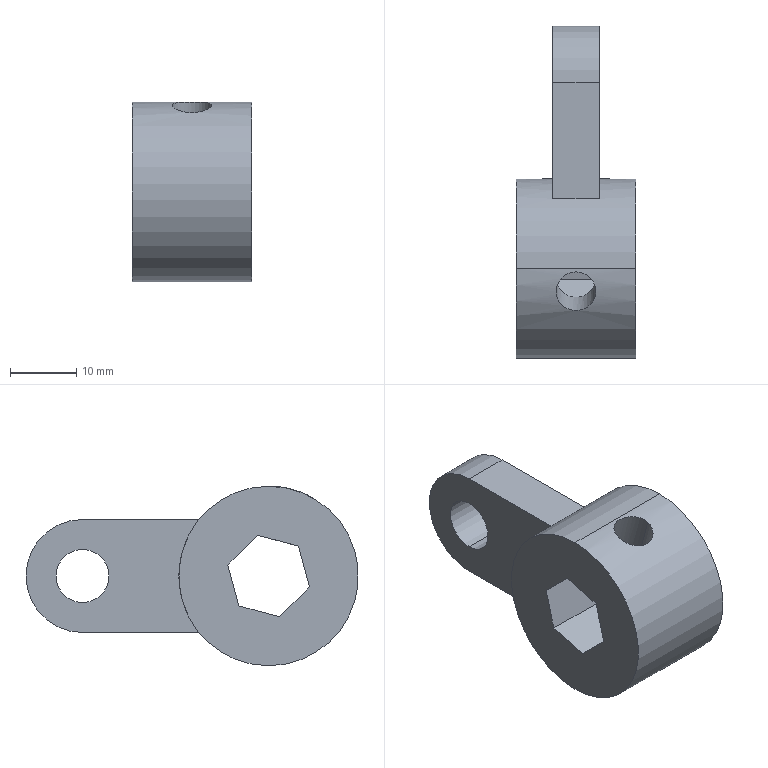Part | NX | features BREP 1 | 1 solid | 19 faces | box 18 x 50 x 27 mm | volume 10478 mm3 | plane 12 | cylinder 7 | commonest cylinder face diameters 6 x2 8 x2 27 x2 17 x1
STEP:
#1=CARTESIAN_POINT('',(-9.,0.,13.5));
#2=VERTEX_POINT('',#1);
#3=CARTESIAN_POINT('',(-9.,0.,-13.5));
#4=VERTEX_POINT('',#3);
#5=CARTESIAN_POINT('',(-9.,0.,0.));
#6=DIRECTION('',(1.,0.,0.));
#7=DIRECTION('',(0.,0.,1.));
#8=AXIS2_PLACEMENT_3D('',#5,#6,#7);
#9=CIRCLE('',#8,13.5);
#10=EDGE_CURVE('',#2,#4,#9,.T.);
#11=ORIENTED_EDGE('',*,*,#10,.F.);
#12=CARTESIAN_POINT('',(-9.,0.,0.));
#13=DIRECTION('',(1.,0.,0.));
#14=DIRECTION('',(0.,0.,-1.));
#15=AXIS2_PLACEMENT_3D('',#12,#13,#14);
#16=CIRCLE('',#15,13.5);
#17=EDGE_CURVE('',#4,#2,#16,.T.);
#18=ORIENTED_EDGE('',*,*,#17,.F.);
#19=EDGE_LOOP('',(#11,#18));
#20=FACE_BOUND('',#19,.T.);
#21=CARTESIAN_POINT('',(-9.,-4.491,4.491));
#22=VERTEX_POINT('',#21);
#23=CARTESIAN_POINT('',(-9.,-6.134,-1.644));
#24=VERTEX_POINT('',#23);
#25=CARTESIAN_POINT('',(-9.,-4.491,4.491));
#26=DIRECTION('',(0.,-0.2588,-0.9659));
#27=VECTOR('',#26,1000.);
#28=LINE('',#25,#27);
#29=EDGE_CURVE('',#22,#24,#28,.T.);
#30=ORIENTED_EDGE('',*,*,#29,.T.);
#31=CARTESIAN_POINT('',(-9.,-1.644,-6.134));
#32=VERTEX_POINT('',#31);
#33=CARTESIAN_POINT('',(-9.,-6.134,-1.644));
#34=DIRECTION('',(0.,0.7071,-0.7071));
#35=VECTOR('',#34,1000.);
#36=LINE('',#33,#35);
#37=EDGE_CURVE('',#24,#32,#36,.T.);
#38=ORIENTED_EDGE('',*,*,#37,.T.);
#39=CARTESIAN_POINT('',(-9.,4.491,-4.491));
#40=VERTEX_POINT('',#39);
#41=CARTESIAN_POINT('',(-9.,-1.644,-6.134));
#42=DIRECTION('',(0.,0.9659,0.2588));
#43=VECTOR('',#42,1000.);
#44=LINE('',#41,#43);
#45=EDGE_CURVE('',#32,#40,#44,.T.);
#46=ORIENTED_EDGE('',*,*,#45,.T.);
#47=CARTESIAN_POINT('',(-9.,6.134,1.644));
#48=VERTEX_POINT('',#47);
#49=CARTESIAN_POINT('',(-9.,4.491,-4.491));
#50=DIRECTION('',(0.,0.2588,0.9659));
#51=VECTOR('',#50,1000.);
#52=LINE('',#49,#51);
#53=EDGE_CURVE('',#40,#48,#52,.T.);
#54=ORIENTED_EDGE('',*,*,#53,.T.);
#55=CARTESIAN_POINT('',(-9.,1.644,6.134));
#56=VERTEX_POINT('',#55);
#57=CARTESIAN_POINT('',(-9.,6.134,1.644));
#58=DIRECTION('',(0.,-0.7071,0.7071));
#59=VECTOR('',#58,1000.);
#60=LINE('',#57,#59);
#61=EDGE_CURVE('',#48,#56,#60,.T.);
#62=ORIENTED_EDGE('',*,*,#61,.T.);
#63=CARTESIAN_POINT('',(-9.,1.644,6.134));
#64=DIRECTION('',(0.,-0.9659,-0.2588));
#65=VECTOR('',#64,1000.);
#66=LINE('',#63,#65);
#67=EDGE_CURVE('',#56,#22,#66,.T.);
#68=ORIENTED_EDGE('',*,*,#67,.T.);
#69=EDGE_LOOP('',(#30,#38,#46,#54,#62,#68));
#70=FACE_BOUND('',#69,.T.);
#71=CARTESIAN_POINT('',(-9.,0.,0.));
#72=DIRECTION('',(1.,0.,0.));
#73=DIRECTION('',(0.,1.,0.));
#74=AXIS2_PLACEMENT_3D('',#71,#72,#73);
#75=PLANE('',#74);
#76=ADVANCED_FACE('',(#20,#70),#75,.F.);
#77=CARTESIAN_POINT('',(9.,0.,13.5));
#78=VERTEX_POINT('',#77);
#79=CARTESIAN_POINT('',(-9.,0.,13.5));
#80=DIRECTION('',(1.,0.,0.));
#81=VECTOR('',#80,1000.);
#82=LINE('',#79,#81);
#83=EDGE_CURVE('',#78,#2,#82,.F.);
#84=ORIENTED_EDGE('',*,*,#83,.F.);
#85=CARTESIAN_POINT('',(9.,0.,-13.5));
#86=VERTEX_POINT('',#85);
#87=CARTESIAN_POINT('',(9.,0.,0.));
#88=DIRECTION('',(1.,0.,0.));
#89=DIRECTION('',(0.,0.,-1.));
#90=AXIS2_PLACEMENT_3D('',#87,#88,#89);
#91=CIRCLE('',#90,13.5);
#92=EDGE_CURVE('',#86,#78,#91,.T.);
#93=ORIENTED_EDGE('',*,*,#92,.F.);
#94=CARTESIAN_POINT('',(-9.,0.,-13.5));
#95=DIRECTION('',(1.,0.,0.));
#96=VECTOR('',#95,1000.);
#97=LINE('',#94,#96);
#98=EDGE_CURVE('',#86,#4,#97,.F.);
#99=ORIENTED_EDGE('',*,*,#98,.T.);
#100=ORIENTED_EDGE('',*,*,#17,.T.);
#101=EDGE_LOOP('',(#84,#93,#99,#100));
#102=FACE_BOUND('',#101,.T.);
#103=CARTESIAN_POINT('',(3.5,10.488,-8.5));
#104=VERTEX_POINT('',#103);
#105=CARTESIAN_POINT('',(3.5,10.488,8.5));
#106=VERTEX_POINT('',#105);
#107=CARTESIAN_POINT('',(3.5,0.,0.));
#108=DIRECTION('',(1.,0.,0.));
#109=DIRECTION('',(0.,0.7769,-0.6296));
#110=AXIS2_PLACEMENT_3D('',#107,#108,#109);
#111=CIRCLE('',#110,13.5);
#112=EDGE_CURVE('',#104,#106,#111,.T.);
#113=ORIENTED_EDGE('',*,*,#112,.T.);
#114=CARTESIAN_POINT('',(-3.5,10.488,8.5));
#115=VERTEX_POINT('',#114);
#116=CARTESIAN_POINT('',(-3.5,10.488,8.5));
#117=DIRECTION('',(1.,0.,0.));
#118=VECTOR('',#117,1000.);
#119=LINE('',#116,#118);
#120=EDGE_CURVE('',#115,#106,#119,.T.);
#121=ORIENTED_EDGE('',*,*,#120,.F.);
#122=CARTESIAN_POINT('',(-3.5,10.488,-8.5));
#123=VERTEX_POINT('',#122);
#124=CARTESIAN_POINT('',(-3.5,0.,0.));
#125=DIRECTION('',(1.,0.,0.));
#126=DIRECTION('',(0.,0.7769,-0.6296));
#127=AXIS2_PLACEMENT_3D('',#124,#125,#126);
#128=CIRCLE('',#127,13.5);
#129=EDGE_CURVE('',#123,#115,#128,.T.);
#130=ORIENTED_EDGE('',*,*,#129,.F.);
#131=CARTESIAN_POINT('',(-3.5,10.488,-8.5));
#132=DIRECTION('',(1.,0.,0.));
#133=VECTOR('',#132,1000.);
#134=LINE('',#131,#133);
#135=EDGE_CURVE('',#123,#104,#134,.T.);
#136=ORIENTED_EDGE('',*,*,#135,.T.);
#137=EDGE_LOOP('',(#113,#121,#130,#136));
#138=FACE_BOUND('',#137,.T.);
#139=CARTESIAN_POINT('',(-9.,0.,0.));
#140=DIRECTION('',(1.,0.,0.));
#141=DIRECTION('',(0.,0.,-1.));
#142=AXIS2_PLACEMENT_3D('',#139,#140,#141);
#143=CYLINDRICAL_SURFACE('',#142,13.5);
#144=ADVANCED_FACE('',(#102,#138),#143,.T.);
#145=ORIENTED_EDGE('',*,*,#98,.F.);
#146=CARTESIAN_POINT('',(9.,0.,0.));
#147=DIRECTION('',(1.,0.,0.));
#148=DIRECTION('',(0.,0.,1.));
#149=AXIS2_PLACEMENT_3D('',#146,#147,#148);
#150=CIRCLE('',#149,13.5);
#151=EDGE_CURVE('',#78,#86,#150,.T.);
#152=ORIENTED_EDGE('',*,*,#151,.F.);
#153=ORIENTED_EDGE('',*,*,#83,.T.);
#154=ORIENTED_EDGE('',*,*,#10,.T.);
#155=EDGE_LOOP('',(#145,#152,#153,#154));
#156=FACE_BOUND('',#155,.T.);
#157=CARTESIAN_POINT('',(-3.,-3.494,13.04));
#158=VERTEX_POINT('',#157);
#159=CARTESIAN_POINT('',(3.,-3.494,13.04));
#160=VERTEX_POINT('',#159);
#161=CARTESIAN_POINT('',(-3.,-3.494,13.04));
#162=CARTESIAN_POINT('',(-3.,-2.73,13.245));
#163=CARTESIAN_POINT('',(-2.352,-1.186,13.486));
#164=CARTESIAN_POINT('',(0.0001371,-0.1703,13.492));
#165=CARTESIAN_POINT('',(2.354,-1.187,13.486));
#166=CARTESIAN_POINT('',(3.,-2.732,13.244));
#167=CARTESIAN_POINT('',(3.,-3.494,13.04));
#168=B_SPLINE_CURVE_WITH_KNOTS('',3,(#161,#162,#163,#164,#165,#166,#167),.UNSPECIFIED.,.F.,.F.,(4,1,1,1,4),(0.,0.25,0.5,0.75,1.),.UNSPECIFIED.);
#169=EDGE_CURVE('',#158,#160,#168,.T.);
#170=ORIENTED_EDGE('',*,*,#169,.T.);
#171=CARTESIAN_POINT('',(3.,-3.494,13.04));
#172=CARTESIAN_POINT('',(3.,-4.258,12.835));
#173=CARTESIAN_POINT('',(2.352,-5.716,12.272));
#174=CARTESIAN_POINT('',(-0.0001371,-6.599,11.77));
#175=CARTESIAN_POINT('',(-2.354,-5.715,12.273));
#176=CARTESIAN_POINT('',(-3.,-4.256,12.836));
#177=CARTESIAN_POINT('',(-3.,-3.494,13.04));
#178=B_SPLINE_CURVE_WITH_KNOTS('',3,(#171,#172,#173,#174,#175,#176,#177),.UNSPECIFIED.,.F.,.F.,(4,1,1,1,4),(0.,0.25,0.5,0.75,1.),.UNSPECIFIED.);
#179=EDGE_CURVE('',#160,#158,#178,.T.);
#180=ORIENTED_EDGE('',*,*,#179,.T.);
#181=EDGE_LOOP('',(#170,#180));
#182=FACE_BOUND('',#181,.T.);
#183=CARTESIAN_POINT('',(-9.,0.,0.));
#184=DIRECTION('',(1.,0.,0.));
#185=DIRECTION('',(0.,0.,-1.));
#186=AXIS2_PLACEMENT_3D('',#183,#184,#185);
#187=CYLINDRICAL_SURFACE('',#186,13.5);
#188=ADVANCED_FACE('',(#156,#182),#187,.T.);
#189=ORIENTED_EDGE('',*,*,#151,.T.);
#190=ORIENTED_EDGE('',*,*,#92,.T.);
#191=EDGE_LOOP('',(#189,#190));
#192=FACE_BOUND('',#191,.T.);
#193=CARTESIAN_POINT('',(9.,6.134,1.644));
#194=VERTEX_POINT('',#193);
#195=CARTESIAN_POINT('',(9.,1.644,6.134));
#196=VERTEX_POINT('',#195);
#197=CARTESIAN_POINT('',(9.,6.134,1.644));
#198=DIRECTION('',(0.,-0.7071,0.7071));
#199=VECTOR('',#198,1000.);
#200=LINE('',#197,#199);
#201=EDGE_CURVE('',#194,#196,#200,.T.);
#202=ORIENTED_EDGE('',*,*,#201,.F.);
#203=CARTESIAN_POINT('',(9.,4.491,-4.491));
#204=VERTEX_POINT('',#203);
#205=CARTESIAN_POINT('',(9.,4.491,-4.491));
#206=DIRECTION('',(0.,0.2588,0.9659));
#207=VECTOR('',#206,1000.);
#208=LINE('',#205,#207);
#209=EDGE_CURVE('',#204,#194,#208,.T.);
#210=ORIENTED_EDGE('',*,*,#209,.F.);
#211=CARTESIAN_POINT('',(9.,-1.644,-6.134));
#212=VERTEX_POINT('',#211);
#213=CARTESIAN_POINT('',(9.,-1.644,-6.134));
#214=DIRECTION('',(0.,0.9659,0.2588));
#215=VECTOR('',#214,1000.);
#216=LINE('',#213,#215);
#217=EDGE_CURVE('',#212,#204,#216,.T.);
#218=ORIENTED_EDGE('',*,*,#217,.F.);
#219=CARTESIAN_POINT('',(9.,-6.134,-1.644));
#220=VERTEX_POINT('',#219);
#221=CARTESIAN_POINT('',(9.,-6.134,-1.644));
#222=DIRECTION('',(0.,0.7071,-0.7071));
#223=VECTOR('',#222,1000.);
#224=LINE('',#221,#223);
#225=EDGE_CURVE('',#220,#212,#224,.T.);
#226=ORIENTED_EDGE('',*,*,#225,.F.);
#227=CARTESIAN_POINT('',(9.,-4.491,4.491));
#228=VERTEX_POINT('',#227);
#229=CARTESIAN_POINT('',(9.,-4.491,4.491));
#230=DIRECTION('',(0.,-0.2588,-0.9659));
#231=VECTOR('',#230,1000.);
#232=LINE('',#229,#231);
#233=EDGE_CURVE('',#228,#220,#232,.T.);
#234=ORIENTED_EDGE('',*,*,#233,.F.);
#235=CARTESIAN_POINT('',(9.,1.644,6.134));
#236=DIRECTION('',(0.,-0.9659,-0.2588));
#237=VECTOR('',#236,1000.);
#238=LINE('',#235,#237);
#239=EDGE_CURVE('',#196,#228,#238,.T.);
#240=ORIENTED_EDGE('',*,*,#239,.F.);
#241=EDGE_LOOP('',(#202,#210,#218,#226,#234,#240));
#242=FACE_BOUND('',#241,.T.);
#243=CARTESIAN_POINT('',(9.,0.,0.));
#244=DIRECTION('',(1.,0.,0.));
#245=DIRECTION('',(0.,1.,0.));
#246=AXIS2_PLACEMENT_3D('',#243,#244,#245);
#247=PLANE('',#246);
#248=ADVANCED_FACE('',(#192,#242),#247,.T.);
#249=CARTESIAN_POINT('',(9.,1.644,6.134));
#250=DIRECTION('',(-1.,0.,0.));
#251=VECTOR('',#250,1000.);
#252=LINE('',#249,#251);
#253=EDGE_CURVE('',#196,#56,#252,.T.);
#254=ORIENTED_EDGE('',*,*,#253,.F.);
#255=ORIENTED_EDGE('',*,*,#239,.T.);
#256=CARTESIAN_POINT('',(9.,-4.491,4.491));
#257=DIRECTION('',(-1.,0.,0.));
#258=VECTOR('',#257,1000.);
#259=LINE('',#256,#258);
#260=EDGE_CURVE('',#228,#22,#259,.T.);
#261=ORIENTED_EDGE('',*,*,#260,.T.);
#262=ORIENTED_EDGE('',*,*,#67,.F.);
#263=EDGE_LOOP('',(#254,#255,#261,#262));
#264=FACE_BOUND('',#263,.T.);
#265=CARTESIAN_POINT('',(-3.,-1.424,5.313));
#266=VERTEX_POINT('',#265);
#267=CARTESIAN_POINT('',(3.,-1.424,5.313));
#268=VERTEX_POINT('',#267);
#269=CARTESIAN_POINT('',(0.,-1.424,5.313));
#270=DIRECTION('',(0.,0.2588,-0.9659));
#271=DIRECTION('',(-1.,0.,0.));
#272=AXIS2_PLACEMENT_3D('',#269,#270,#271);
#273=CIRCLE('',#272,3.);
#274=EDGE_CURVE('',#266,#268,#273,.T.);
#275=ORIENTED_EDGE('',*,*,#274,.F.);
#276=CARTESIAN_POINT('',(0.,-1.424,5.313));
#277=DIRECTION('',(0.,0.2588,-0.9659));
#278=DIRECTION('',(1.,0.,0.));
#279=AXIS2_PLACEMENT_3D('',#276,#277,#278);
#280=CIRCLE('',#279,3.);
#281=EDGE_CURVE('',#268,#266,#280,.T.);
#282=ORIENTED_EDGE('',*,*,#281,.F.);
#283=EDGE_LOOP('',(#275,#282));
#284=FACE_BOUND('',#283,.T.);
#285=CARTESIAN_POINT('',(10.8,1.644,6.134));
#286=DIRECTION('',(0.,-0.2588,0.9659));
#287=DIRECTION('',(-1.,0.,0.));
#288=AXIS2_PLACEMENT_3D('',#285,#286,#287);
#289=PLANE('',#288);
#290=ADVANCED_FACE('',(#264,#284),#289,.F.);
#291=ORIENTED_EDGE('',*,*,#260,.F.);
#292=ORIENTED_EDGE('',*,*,#233,.T.);
#293=CARTESIAN_POINT('',(9.,-6.134,-1.644));
#294=DIRECTION('',(-1.,0.,0.));
#295=VECTOR('',#294,1000.);
#296=LINE('',#293,#295);
#297=EDGE_CURVE('',#220,#24,#296,.T.);
#298=ORIENTED_EDGE('',*,*,#297,.T.);
#299=ORIENTED_EDGE('',*,*,#29,.F.);
#300=EDGE_LOOP('',(#291,#292,#298,#299));
#301=FACE_BOUND('',#300,.T.);
#302=CARTESIAN_POINT('',(10.8,-4.491,4.491));
#303=DIRECTION('',(0.,-0.9659,0.2588));
#304=DIRECTION('',(-1.,0.,0.));
#305=AXIS2_PLACEMENT_3D('',#302,#303,#304);
#306=PLANE('',#305);
#307=ADVANCED_FACE('',(#301),#306,.F.);
#308=ORIENTED_EDGE('',*,*,#297,.F.);
#309=ORIENTED_EDGE('',*,*,#225,.T.);
#310=CARTESIAN_POINT('',(9.,-1.644,-6.134));
#311=DIRECTION('',(-1.,0.,0.));
#312=VECTOR('',#311,1000.);
#313=LINE('',#310,#312);
#314=EDGE_CURVE('',#212,#32,#313,.T.);
#315=ORIENTED_EDGE('',*,*,#314,.T.);
#316=ORIENTED_EDGE('',*,*,#37,.F.);
#317=EDGE_LOOP('',(#308,#309,#315,#316));
#318=FACE_BOUND('',#317,.T.);
#319=CARTESIAN_POINT('',(10.8,-6.134,-1.644));
#320=DIRECTION('',(0.,-0.7071,-0.7071));
#321=DIRECTION('',(0.,-0.7071,0.7071));
#322=AXIS2_PLACEMENT_3D('',#319,#320,#321);
#323=PLANE('',#322);
#324=ADVANCED_FACE('',(#318),#323,.F.);
#325=ORIENTED_EDGE('',*,*,#314,.F.);
#326=ORIENTED_EDGE('',*,*,#217,.T.);
#327=CARTESIAN_POINT('',(9.,4.491,-4.491));
#328=DIRECTION('',(-1.,0.,0.));
#329=VECTOR('',#328,1000.);
#330=LINE('',#327,#329);
#331=EDGE_CURVE('',#204,#40,#330,.T.);
#332=ORIENTED_EDGE('',*,*,#331,.T.);
#333=ORIENTED_EDGE('',*,*,#45,.F.);
#334=EDGE_LOOP('',(#325,#326,#332,#333));
#335=FACE_BOUND('',#334,.T.);
#336=CARTESIAN_POINT('',(10.8,-1.644,-6.134));
#337=DIRECTION('',(0.,0.2588,-0.9659));
#338=DIRECTION('',(-1.,0.,0.));
#339=AXIS2_PLACEMENT_3D('',#336,#337,#338);
#340=PLANE('',#339);
#341=ADVANCED_FACE('',(#335),#340,.F.);
#342=ORIENTED_EDGE('',*,*,#331,.F.);
#343=ORIENTED_EDGE('',*,*,#209,.T.);
#344=CARTESIAN_POINT('',(9.,6.134,1.644));
#345=DIRECTION('',(-1.,0.,0.));
#346=VECTOR('',#345,1000.);
#347=LINE('',#344,#346);
#348=EDGE_CURVE('',#194,#48,#347,.T.);
#349=ORIENTED_EDGE('',*,*,#348,.T.);
#350=ORIENTED_EDGE('',*,*,#53,.F.);
#351=EDGE_LOOP('',(#342,#343,#349,#350));
#352=FACE_BOUND('',#351,.T.);
#353=CARTESIAN_POINT('',(10.8,4.491,-4.491));
#354=DIRECTION('',(0.,0.9659,-0.2588));
#355=DIRECTION('',(-1.,0.,0.));
#356=AXIS2_PLACEMENT_3D('',#353,#354,#355);
#357=PLANE('',#356);
#358=ADVANCED_FACE('',(#352),#357,.F.);
#359=ORIENTED_EDGE('',*,*,#348,.F.);
#360=ORIENTED_EDGE('',*,*,#201,.T.);
#361=ORIENTED_EDGE('',*,*,#253,.T.);
#362=ORIENTED_EDGE('',*,*,#61,.F.);
#363=EDGE_LOOP('',(#359,#360,#361,#362));
#364=FACE_BOUND('',#363,.T.);
#365=CARTESIAN_POINT('',(10.8,6.134,1.644));
#366=DIRECTION('',(0.,0.7071,0.7071));
#367=DIRECTION('',(1.,0.,0.));
#368=AXIS2_PLACEMENT_3D('',#365,#366,#367);
#369=PLANE('',#368);
#370=ADVANCED_FACE('',(#364),#369,.F.);
#371=CARTESIAN_POINT('',(3.,-1.424,5.313));
#372=DIRECTION('',(0.,-0.2588,0.9659));
#373=VECTOR('',#372,1000.);
#374=LINE('',#371,#373);
#375=EDGE_CURVE('',#160,#268,#374,.F.);
#376=ORIENTED_EDGE('',*,*,#375,.T.);
#377=ORIENTED_EDGE('',*,*,#281,.T.);
#378=CARTESIAN_POINT('',(-3.,-1.424,5.313));
#379=DIRECTION('',(0.,-0.2588,0.9659));
#380=VECTOR('',#379,1000.);
#381=LINE('',#378,#380);
#382=EDGE_CURVE('',#158,#266,#381,.F.);
#383=ORIENTED_EDGE('',*,*,#382,.F.);
#384=ORIENTED_EDGE('',*,*,#179,.F.);
#385=EDGE_LOOP('',(#376,#377,#383,#384));
#386=FACE_BOUND('',#385,.T.);
#387=CARTESIAN_POINT('',(0.,-1.424,5.313));
#388=DIRECTION('',(0.,0.2588,-0.9659));
#389=DIRECTION('',(1.,0.,0.));
#390=AXIS2_PLACEMENT_3D('',#387,#388,#389);
#391=CYLINDRICAL_SURFACE('',#390,3.);
#392=ADVANCED_FACE('',(#386),#391,.F.);
#393=ORIENTED_EDGE('',*,*,#382,.T.);
#394=ORIENTED_EDGE('',*,*,#274,.T.);
#395=ORIENTED_EDGE('',*,*,#375,.F.);
#396=ORIENTED_EDGE('',*,*,#169,.F.);
#397=EDGE_LOOP('',(#393,#394,#395,#396));
#398=FACE_BOUND('',#397,.T.);
#399=CARTESIAN_POINT('',(0.,-1.424,5.313));
#400=DIRECTION('',(0.,0.2588,-0.9659));
#401=DIRECTION('',(1.,0.,0.));
#402=AXIS2_PLACEMENT_3D('',#399,#400,#401);
#403=CYLINDRICAL_SURFACE('',#402,3.);
#404=ADVANCED_FACE('',(#398),#403,.F.);
#405=CARTESIAN_POINT('',(-3.5,28.,-8.5));
#406=VERTEX_POINT('',#405);
#407=CARTESIAN_POINT('',(-3.5,10.488,-8.5));
#408=DIRECTION('',(0.,1.,0.));
#409=VECTOR('',#408,1000.);
#410=LINE('',#407,#409);
#411=EDGE_CURVE('',#123,#406,#410,.T.);
#412=ORIENTED_EDGE('',*,*,#411,.T.);
#413=CARTESIAN_POINT('',(3.5,28.,-8.5));
#414=VERTEX_POINT('',#413);
#415=CARTESIAN_POINT('',(-3.5,28.,-8.5));
#416=DIRECTION('',(1.,0.,0.));
#417=VECTOR('',#416,1000.);
#418=LINE('',#415,#417);
#419=EDGE_CURVE('',#406,#414,#418,.T.);
#420=ORIENTED_EDGE('',*,*,#419,.T.);
#421=CARTESIAN_POINT('',(3.5,10.488,-8.5));
#422=DIRECTION('',(0.,1.,0.));
#423=VECTOR('',#422,1000.);
#424=LINE('',#421,#423);
#425=EDGE_CURVE('',#104,#414,#424,.T.);
#426=ORIENTED_EDGE('',*,*,#425,.F.);
#427=ORIENTED_EDGE('',*,*,#135,.F.);
#428=EDGE_LOOP('',(#412,#420,#426,#427));
#429=FACE_BOUND('',#428,.T.);
#430=CARTESIAN_POINT('',(-3.5,10.488,-8.5));
#431=DIRECTION('',(0.,0.,-1.));
#432=DIRECTION('',(0.,-1.,0.));
#433=AXIS2_PLACEMENT_3D('',#430,#431,#432);
#434=PLANE('',#433);
#435=ADVANCED_FACE('',(#429),#434,.T.);
#436=ORIENTED_EDGE('',*,*,#425,.T.);
#437=CARTESIAN_POINT('',(3.5,28.,8.5));
#438=VERTEX_POINT('',#437);
#439=CARTESIAN_POINT('',(3.5,28.,0.));
#440=DIRECTION('',(1.,0.,0.));
#441=DIRECTION('',(0.,0.,-1.));
#442=AXIS2_PLACEMENT_3D('',#439,#440,#441);
#443=CIRCLE('',#442,8.5);
#444=EDGE_CURVE('',#414,#438,#443,.T.);
#445=ORIENTED_EDGE('',*,*,#444,.T.);
#446=CARTESIAN_POINT('',(3.5,28.,8.5));
#447=DIRECTION('',(0.,-1.,0.));
#448=VECTOR('',#447,1000.);
#449=LINE('',#446,#448);
#450=EDGE_CURVE('',#438,#106,#449,.T.);
#451=ORIENTED_EDGE('',*,*,#450,.T.);
#452=ORIENTED_EDGE('',*,*,#112,.F.);
#453=EDGE_LOOP('',(#436,#445,#451,#452));
#454=FACE_BOUND('',#453,.T.);
#455=CARTESIAN_POINT('',(3.5,28.,4.));
#456=VERTEX_POINT('',#455);
#457=CARTESIAN_POINT('',(3.5,28.,-4.));
#458=VERTEX_POINT('',#457);
#459=CARTESIAN_POINT('',(3.5,28.,0.));
#460=DIRECTION('',(1.,0.,0.));
#461=DIRECTION('',(0.,0.,1.));
#462=AXIS2_PLACEMENT_3D('',#459,#460,#461);
#463=CIRCLE('',#462,4.);
#464=EDGE_CURVE('',#456,#458,#463,.T.);
#465=ORIENTED_EDGE('',*,*,#464,.F.);
#466=CARTESIAN_POINT('',(3.5,28.,0.));
#467=DIRECTION('',(1.,0.,0.));
#468=DIRECTION('',(0.,0.,-1.));
#469=AXIS2_PLACEMENT_3D('',#466,#467,#468);
#470=CIRCLE('',#469,4.);
#471=EDGE_CURVE('',#458,#456,#470,.T.);
#472=ORIENTED_EDGE('',*,*,#471,.F.);
#473=EDGE_LOOP('',(#465,#472));
#474=FACE_BOUND('',#473,.T.);
#475=CARTESIAN_POINT('',(3.5,0.,0.));
#476=DIRECTION('',(1.,0.,0.));
#477=DIRECTION('',(0.,1.,0.));
#478=AXIS2_PLACEMENT_3D('',#475,#476,#477);
#479=PLANE('',#478);
#480=ADVANCED_FACE('',(#454,#474),#479,.T.);
#481=ORIENTED_EDGE('',*,*,#450,.F.);
#482=CARTESIAN_POINT('',(-3.5,28.,8.5));
#483=VERTEX_POINT('',#482);
#484=CARTESIAN_POINT('',(-3.5,28.,8.5));
#485=DIRECTION('',(1.,0.,0.));
#486=VECTOR('',#485,1000.);
#487=LINE('',#484,#486);
#488=EDGE_CURVE('',#483,#438,#487,.T.);
#489=ORIENTED_EDGE('',*,*,#488,.F.);
#490=CARTESIAN_POINT('',(-3.5,28.,8.5));
#491=DIRECTION('',(0.,-1.,0.));
#492=VECTOR('',#491,1000.);
#493=LINE('',#490,#492);
#494=EDGE_CURVE('',#483,#115,#493,.T.);
#495=ORIENTED_EDGE('',*,*,#494,.T.);
#496=ORIENTED_EDGE('',*,*,#120,.T.);
#497=EDGE_LOOP('',(#481,#489,#495,#496));
#498=FACE_BOUND('',#497,.T.);
#499=CARTESIAN_POINT('',(-3.5,28.,8.5));
#500=DIRECTION('',(0.,0.,1.));
#501=DIRECTION('',(1.,0.,0.));
#502=AXIS2_PLACEMENT_3D('',#499,#500,#501);
#503=PLANE('',#502);
#504=ADVANCED_FACE('',(#498),#503,.T.);
#505=ORIENTED_EDGE('',*,*,#494,.F.);
#506=CARTESIAN_POINT('',(-3.5,28.,0.));
#507=DIRECTION('',(1.,0.,0.));
#508=DIRECTION('',(0.,0.,-1.));
#509=AXIS2_PLACEMENT_3D('',#506,#507,#508);
#510=CIRCLE('',#509,8.5);
#511=EDGE_CURVE('',#406,#483,#510,.T.);
#512=ORIENTED_EDGE('',*,*,#511,.F.);
#513=ORIENTED_EDGE('',*,*,#411,.F.);
#514=ORIENTED_EDGE('',*,*,#129,.T.);
#515=EDGE_LOOP('',(#505,#512,#513,#514));
#516=FACE_BOUND('',#515,.T.);
#517=CARTESIAN_POINT('',(-3.5,28.,4.));
#518=VERTEX_POINT('',#517);
#519=CARTESIAN_POINT('',(-3.5,28.,-4.));
#520=VERTEX_POINT('',#519);
#521=CARTESIAN_POINT('',(-3.5,28.,0.));
#522=DIRECTION('',(1.,0.,0.));
#523=DIRECTION('',(0.,0.,1.));
#524=AXIS2_PLACEMENT_3D('',#521,#522,#523);
#525=CIRCLE('',#524,4.);
#526=EDGE_CURVE('',#518,#520,#525,.T.);
#527=ORIENTED_EDGE('',*,*,#526,.T.);
#528=CARTESIAN_POINT('',(-3.5,28.,0.));
#529=DIRECTION('',(1.,0.,0.));
#530=DIRECTION('',(0.,0.,-1.));
#531=AXIS2_PLACEMENT_3D('',#528,#529,#530);
#532=CIRCLE('',#531,4.);
#533=EDGE_CURVE('',#520,#518,#532,.T.);
#534=ORIENTED_EDGE('',*,*,#533,.T.);
#535=EDGE_LOOP('',(#527,#534));
#536=FACE_BOUND('',#535,.T.);
#537=CARTESIAN_POINT('',(-3.5,0.,0.));
#538=DIRECTION('',(1.,0.,0.));
#539=DIRECTION('',(0.,1.,0.));
#540=AXIS2_PLACEMENT_3D('',#537,#538,#539);
#541=PLANE('',#540);
#542=ADVANCED_FACE('',(#516,#536),#541,.F.);
#543=ORIENTED_EDGE('',*,*,#488,.T.);
#544=ORIENTED_EDGE('',*,*,#444,.F.);
#545=ORIENTED_EDGE('',*,*,#419,.F.);
#546=ORIENTED_EDGE('',*,*,#511,.T.);
#547=EDGE_LOOP('',(#543,#544,#545,#546));
#548=FACE_BOUND('',#547,.T.);
#549=CARTESIAN_POINT('',(-3.5,28.,0.));
#550=DIRECTION('',(1.,0.,0.));
#551=DIRECTION('',(0.,0.,-1.));
#552=AXIS2_PLACEMENT_3D('',#549,#550,#551);
#553=CYLINDRICAL_SURFACE('',#552,8.5);
#554=ADVANCED_FACE('',(#548),#553,.T.);
#555=CARTESIAN_POINT('',(3.5,28.,-4.));
#556=DIRECTION('',(-1.,0.,0.));
#557=VECTOR('',#556,1000.);
#558=LINE('',#555,#557);
#559=EDGE_CURVE('',#458,#520,#558,.T.);
#560=ORIENTED_EDGE('',*,*,#559,.F.);
#561=ORIENTED_EDGE('',*,*,#471,.T.);
#562=CARTESIAN_POINT('',(3.5,28.,4.));
#563=DIRECTION('',(-1.,0.,0.));
#564=VECTOR('',#563,1000.);
#565=LINE('',#562,#564);
#566=EDGE_CURVE('',#456,#518,#565,.T.);
#567=ORIENTED_EDGE('',*,*,#566,.T.);
#568=ORIENTED_EDGE('',*,*,#533,.F.);
#569=EDGE_LOOP('',(#560,#561,#567,#568));
#570=FACE_BOUND('',#569,.T.);
#571=CARTESIAN_POINT('',(10.8,28.,0.));
#572=DIRECTION('',(1.,0.,0.));
#573=DIRECTION('',(0.,0.,-1.));
#574=AXIS2_PLACEMENT_3D('',#571,#572,#573);
#575=CYLINDRICAL_SURFACE('',#574,4.);
#576=ADVANCED_FACE('',(#570),#575,.F.);
#577=ORIENTED_EDGE('',*,*,#566,.F.);
#578=ORIENTED_EDGE('',*,*,#464,.T.);
#579=ORIENTED_EDGE('',*,*,#559,.T.);
#580=ORIENTED_EDGE('',*,*,#526,.F.);
#581=EDGE_LOOP('',(#577,#578,#579,#580));
#582=FACE_BOUND('',#581,.T.);
#583=CARTESIAN_POINT('',(10.8,28.,0.));
#584=DIRECTION('',(1.,0.,0.));
#585=DIRECTION('',(0.,0.,-1.));
#586=AXIS2_PLACEMENT_3D('',#583,#584,#585);
#587=CYLINDRICAL_SURFACE('',#586,4.);
#588=ADVANCED_FACE('',(#582),#587,.F.);
#589=CLOSED_SHELL('',(#76,#144,#188,#248,#290,#307,#324,#341,#358,#370,#392,#404,#435,#480,#504,#542,#554,#576,#588));
#590=MANIFOLD_SOLID_BREP('',#589);
#591=(LENGTH_UNIT()NAMED_UNIT(*)SI_UNIT(.MILLI.,.METRE.));
#592=UNCERTAINTY_MEASURE_WITH_UNIT(LENGTH_MEASURE(0.0508),#591,'','');
#593=(NAMED_UNIT(*)PLANE_ANGLE_UNIT()SI_UNIT($,.RADIAN.));
#594=(NAMED_UNIT(*)SI_UNIT($,.STERADIAN.)SOLID_ANGLE_UNIT());
#595=(GEOMETRIC_REPRESENTATION_CONTEXT(3)GLOBAL_UNCERTAINTY_ASSIGNED_CONTEXT((#592))GLOBAL_UNIT_ASSIGNED_CONTEXT((#591,#593,#594))REPRESENTATION_CONTEXT('',''));
#596=ADVANCED_BREP_SHAPE_REPRESENTATION('',(#590),#595);